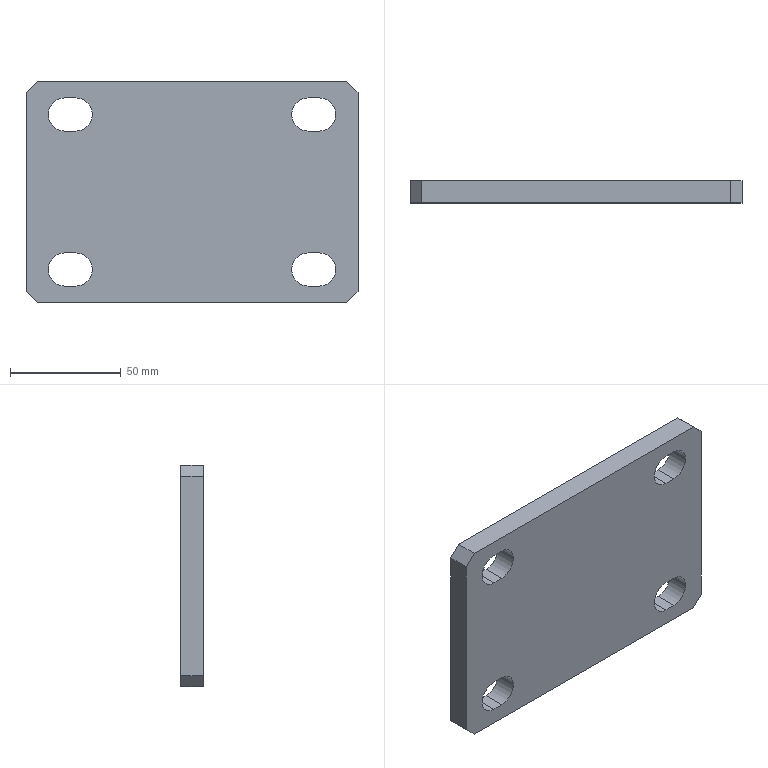Part | STEP file | E3-楼梯立柱连接Plate 1 | 1 solid | 26 faces | box 150 x 10 x 100 mm | volume 139431 mm3 | plane 18 | cylinder 8 | commonest cylinder face diameters 15 x8